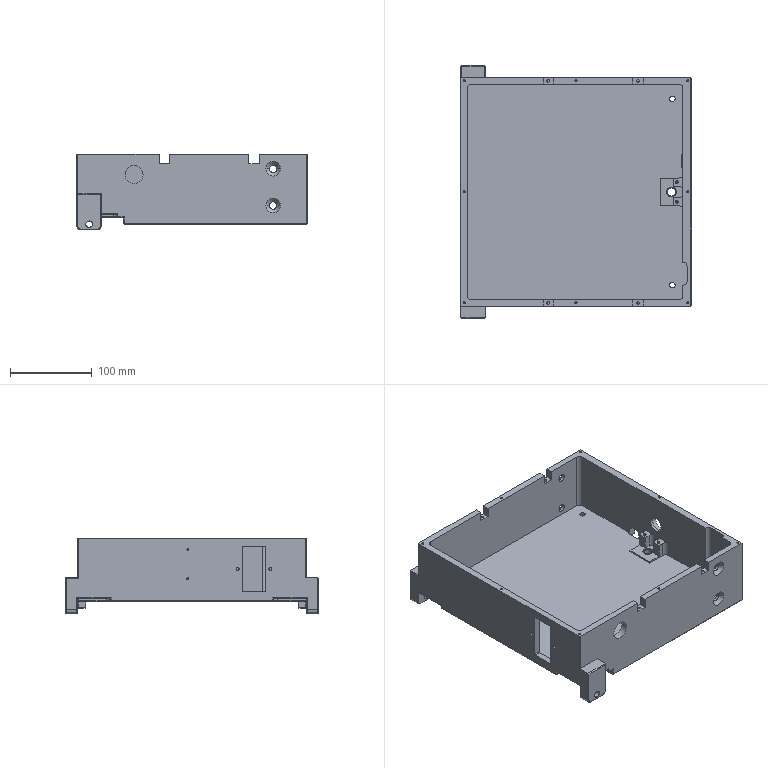CAM job | Mastercam | 3-axis milling, 5-axis milling, drilling
Tools:
tool_number,name,type,diameter_mm,corner_radius_mm,flutes,flute_length_mm,overall_length_mm,shoulder_length_mm,holder_diameter_mm,length_offset,diameter_offset,default_rpm,default_feed_mm_min,default_plunge_mm_min,coolant
1,6 Chamfer Mill,chamfer mill,6,0,4,25,75,30,50,1,1,4167,500.04,600,COOL_OFF
2,2 Flat End Mill,end mill,2,0,4,25,75,25,50,2,2,5000,600,600,COOL_OFF
4,4 Ball Mill / Bull Nose Mill,ball end mill,4,2,4,25,100,30,50,4,4,3000,360,600,COOL_OFF
5,5 Flat End Mill,end mill,5,0,4,25,75,25,50,5,5,2000,240,600,COOL_OFF
6,6 Flat End Mill,end mill,6,0,4,25,75,25,50,6,6,1667,200.04,600,COOL_OFF
7,6 Chamfer Mill,chamfer mill,6,0,4,25,75,30,50,7,7,4167,500.04,600,COOL_OFF
10,10 Flat End Mill,end mill,10,0,4,25,75,25,50,10,10,1000,120,600,COOL_OFF
11,10 Flat End Mill,end mill,10,0,4,25,75,25,50,11,11,1000,120,600,COOL_OFF
12,12 Flat End Mill,end mill,12,0,4,25,75,25,50,12,12,833,99.96,600,COOL_OFF
15,6 Bull Nose Mill,bull end mill,6,1,4,25,100,25,50,15,15,2000,240,600,COOL_OFF
20,20 Flat End Mill,end mill,20,0,4,100,100,100,50,20,20,500,60,600,COOL_OFF
23,50 Flat End Mill,end mill,50,0,4,25,75,25,50,23,23,200,24,600,COOL_OFF
24,100 Flat End Mill,end mill,100,0,4,25,75,25,50,24,24,100,12,600,COOL_OFF
Operations:
seq,operation,operation_type,tool_number,tool_name,tool_diameter_mm,spindle_rpm,feed_mm_min,plunge_mm_min,retract_mm_min,cycle_time_s,wcs,posted,nc_file
1,Facing - [WCS: Plane] - [Tplane: Plane],Facing,24,100 Flat End Mill,100,4000,1200,600,1200,129.734,Plane,yes,.nc
2,Contour (Ramp) - [WCS: Plane] - [Tplane: Plane],Contour,23,50 Flat End Mill,50,4000,4000,600,1200,942.056,Plane,yes,.nc
3,Contour (Ramp) - [WCS: Plane] - [Tplane: Plane],Contour,23,50 Flat End Mill,50,4000,4000,600,1200,945.196,Plane,yes,.nc
4,3D High Speed (Area roughing) - [WCS: Plane] - [Tplane: Plane],HighSpeed3D,23,50 Flat End Mill,50,4000,4000,600,1200,2549.3,Plane,yes,.nc
5,3D High Speed (Waterline rest passes) - [WCS: Plane] - [Tplane: Plane],HighSpeed3D,20,20 Flat End Mill,20,4000,4000,600,1200,319.738,Plane,yes,.nc
6,Contour (Ramp) - [WCS: Plane] - [Tplane: Plane],Contour,10,10 Flat End Mill,10,7000,3000,600,1200,74.419,Plane,yes,.nc
7,Contour (2D) - [WCS: Plane] - [Tplane: Plane],Contour,10,10 Flat End Mill,10,7000,1000,600,1200,25.222,Plane,yes,.nc
8,Contour (2D) - [WCS: Plane] - [Tplane: Plane],Contour,20,20 Flat End Mill,20,4000,2000,600,1200,157.383,Plane,yes,.nc
9,Contour (Remachining) - [WCS: Plane] - [Tplane: Plane],Contour,20,20 Flat End Mill,20,4000,4000,600,1200,81.306,Plane,yes,.nc
10,Contour (2D) - [WCS: Plane] - [Tplane: Plane],Contour,20,20 Flat End Mill,20,4000,2000,600,1200,163.926,Plane,yes,.nc
11,Contour (Remachining) - [WCS: Plane] - [Tplane: Plane],Contour,10,10 Flat End Mill,10,6500,3500,600,1200,145.198,Plane,yes,.nc
12,Contour (2D) - [WCS: Plane] - [Tplane: Plane],Contour,10,10 Flat End Mill,10,6500,1000,600,1200,497.497,Plane,yes,.nc
13,3D High Speed (Waterline rest passes) - [WCS: Plane] - [Tplane: Plane],HighSpeed3D,11,10 Flat End Mill,10,5500,3000,600,1200,255.251,Plane,yes,.nc
14,Contour (2D) - [WCS: Plane] - [Tplane: Plane],Contour,11,10 Flat End Mill,10,5500,1000,600,1200,124.5,Plane,yes,.nc
15,Contour (2D) - [WCS: Plane] - [Tplane: Plane],Contour,11,10 Flat End Mill,10,5500,1000,600,1200,4.343,Plane,yes,.nc
16,2D High Speed (2D Area Mill) - [WCS: Plane] - [Tplane: Plane],HighSpeed2D,11,10 Flat End Mill,10,5500,1000,600,1200,13.176,Plane,yes,.nc
17,Contour (2D) - [WCS: Plane] - [Tplane: Plane],Contour,11,10 Flat End Mill,10,5500,1000,600,1200,22.528,Plane,yes,.nc
18,Contour (2D) - [WCS: Plane] - [Tplane: Plane],Contour,11,10 Flat End Mill,10,5500,1000,600,1200,261.23,Plane,yes,.nc
19,2D High Speed (2D Area Mill) - [WCS: Plane] - [Tplane: Plane],HighSpeed2D,11,10 Flat End Mill,10,5500,1000,600,1200,742.916,Plane,yes,.nc
20,Drill/Counterbore - [WCS: Plane] - [Tplane: Plane],Drill,1,6 Chamfer Mill,6,5000,200,600,1200,15.45,Plane,yes,.nc
21,Contour (2D chamfer) - [WCS: Plane] - [Tplane: Plane],Contour,7,6 Chamfer Mill,6,6000,1200,600,1200,110.416,Plane,yes,.nc
22,Contour (2D chamfer) - [WCS: Plane] - [Tplane: Plane],Contour,7,6 Chamfer Mill,6,6000,1200,600,1200,11.672,Plane,yes,.nc
23,Contour (2D chamfer) - [WCS: Plane] - [Tplane: Plane],Contour,7,6 Chamfer Mill,6,6000,1200,600,1200,15.232,Plane,yes,.nc
24,Facing - [WCS: Plane-1] - [Tplane: Plane-1],Facing,24,100 Flat End Mill,100,4000,2500,600,1200,1022.912,Plane-1,yes,.nc
25,Contour (2D chamfer) - [WCS: Plane-1] - [Tplane: Plane-1],Contour,7,6 Chamfer Mill,6,6000,1200,600,1200,59.589,Plane-1,yes,.nc
26,Manual Entry (G90G54G0X-300.),ManualEntry,,,,0,0,0,0,0,Plane-2,yes,.nc
27,Contour (Ramp) - [WCS: Plane-2] - [Tplane: Plane-2],Contour,10,10 Flat End Mill,10,7000,2500,600,1200,80.177,Plane-2,yes,.nc
28,Manual Entry (G90G54G0X-300.),ManualEntry,,,,0,0,0,0,0,Plane-2,yes,.nc
29,Contour (Remachining) - [WCS: Plane-2] - [Tplane: Plane-2],Contour,2,2 Flat End Mill,2,6000,2000,600,1200,48.112,Plane-2,yes,.nc
30,Contour (Remachining) - [WCS: Plane-2] - [Tplane: Plane-2],Contour,2,2 Flat End Mill,2,6000,500,600,1200,29.929,Plane-2,yes,.nc
31,Manual Entry (G90G54G0X-300.),ManualEntry,,,,0,0,0,0,0,Plane-2,yes,.nc
32,Contour (2D) - [WCS: Plane-2] - [Tplane: Plane-2],Contour,10,10 Flat End Mill,10,7000,1000,600,1200,8.573,Plane-2,yes,.nc
33,Manual Entry (G90G54G0X-300.),ManualEntry,,,,0,0,0,0,0,Plane-2,yes,.nc
34,Drill/Counterbore - [WCS: Plane-2] - [Tplane: Plane-2],Drill,7,6 Chamfer Mill,6,6000,200,600,1200,3.954,Plane-2,yes,.nc
35,Contour (2D chamfer) - [WCS: Plane-2] - [Tplane: Plane-2],Contour,7,6 Chamfer Mill,6,6000,1000,600,1200,10.508,Plane-2,yes,.nc
36,Manual Entry (G90G54G0X-300.),ManualEntry,,,,0,0,0,0,0,Plane-3,yes,.nc
37,Contour (Ramp) - [WCS: Plane-3] - [Tplane: Plane-3],Contour,10,10 Flat End Mill,10,7000,3000,600,1200,55.331,Plane-3,yes,.nc
38,Contour (2D) - [WCS: Plane-3] - [Tplane: Plane-3],Contour,10,10 Flat End Mill,10,7000,1000,600,1200,10.238,Plane-3,yes,.nc
39,Contour (Ramp) - [WCS: Plane-3] - [Tplane: Plane-3],Contour,10,10 Flat End Mill,10,7000,2500,600,1200,13.576,Plane-3,yes,.nc
40,Contour (Ramp) - [WCS: Plane-3] - [Tplane: Plane-3],Contour,10,10 Flat End Mill,10,7000,3000,600,1200,6.513,Plane-3,yes,.nc
41,Contour (2D) - [WCS: Plane-3] - [Tplane: Plane-3],Contour,10,10 Flat End Mill,10,7000,1000,600,1200,3.526,Plane-3,yes,.nc
42,Manual Entry (fbe),ManualEntry,,,,0,0,0,0,0,Plane-3,yes,.nc
43,Contour (2D) - [WCS: Plane-3] - [Tplane: Plane-3],Contour,10,10 Flat End Mill,10,7000,1000,600,1200,6.461,Plane-3,yes,.nc
44,Manual Entry (G90G54G0X-300.),ManualEntry,,,,0,0,0,0,0,Plane-3,yes,.nc
45,Contour (Ramp) - [WCS: Plane-3] - [Tplane: Plane-3],Contour,6,6 Flat End Mill,6,6500,2500,600,1200,12.033,Plane-3,yes,.nc
46,Contour (2D) - [WCS: Plane-3] - [Tplane: Plane-3],Contour,6,6 Flat End Mill,6,6500,1000,600,1200,3.861,Plane-3,yes,.nc
47,Manual Entry (G90G54G0X-300.),ManualEntry,,,,0,0,0,0,0,Plane-3,yes,.nc
48,Contour (2D chamfer) - [WCS: Plane-3] - [Tplane: Plane-3],Contour,7,6 Chamfer Mill,6,6000,1000,600,1200,19.128,Plane-3,yes,.nc
49,Contour (2D chamfer) - [WCS: Plane-3] - [Tplane: Plane-3],Contour,7,6 Chamfer Mill,6,6000,1000,600,1200,8.572,Plane-3,yes,.nc
50,Drill/Counterbore - [WCS: Plane-3] - [Tplane: Plane-3],Drill,7,6 Chamfer Mill,6,6000,200,600,1200,2.966,Plane-3,yes,.nc
51,Manual Entry (G90G54G0X-300.),ManualEntry,,,,0,0,0,0,0,Plane-3,yes,.nc
52,Contour (Ramp) - [WCS: Plane-4] - [Tplane: Plane-4],Contour,12,12 Flat End Mill,12,7000,3000,600,1200,29.857,Plane-4,yes,.nc
53,Contour (Ramp) - [WCS: Plane-4] - [Tplane: Plane-4],Contour,12,12 Flat End Mill,12,7000,3000,600,1200,19.423,Plane-4,yes,.nc
54,Contour (2D) - [WCS: Plane-4] - [Tplane: Plane-4],Contour,12,12 Flat End Mill,12,7000,1000,600,1200,13.482,Plane-4,yes,.nc
55,Manual Entry (G90G54G0X-300.),ManualEntry,,,,0,0,0,0,0,Plane-3,yes,.nc
56,Contour (Ramp) - [WCS: Plane-4] - [Tplane: Plane-4],Contour,5,5 Flat End Mill,5,7000,2500,600,1200,14.495,Plane-4,yes,.nc
57,Contour (Ramp) - [WCS: Plane-4] - [Tplane: Plane-4],Contour,5,5 Flat End Mill,5,7000,1000,600,1200,5.98,Plane-4,yes,.nc
58,Contour (Ramp) - [WCS: Plane-4] - [Tplane: Plane-4],Contour,5,5 Flat End Mill,5,7000,2000,600,1200,11.785,Plane-4,yes,.nc
59,Contour (Ramp) - [WCS: Plane-4] - [Tplane: Plane-4],Contour,5,5 Flat End Mill,5,7000,1000,600,1200,6.231,Plane-4,yes,.nc
60,Manual Entry (G90G54G0X-300.),ManualEntry,,,,0,0,0,0,0,Plane-3,yes,.nc
61,Surface Finish Flowline - [WCS: Plane-4] - [Tplane: Plane-4],MultiSurfaceFinishFlowline,15,6 Bull Nose Mill,6,7000,3000,600,1200,71.4,Plane-4,yes,.nc
62,Manual Entry (G90G54G0X-300.),ManualEntry,,,,0,0,0,0,0,Plane-3,yes,.nc
63,Contour (2D chamfer) - [WCS: Plane-4] - [Tplane: Plane-4],Contour,7,6 Chamfer Mill,6,6000,1000,600,1200,19.072,Plane-4,yes,.nc
64,Contour (2D chamfer) - [WCS: Plane-4] - [Tplane: Plane-4],Contour,7,6 Chamfer Mill,6,6000,1000,600,1200,2.137,Plane-4,yes,.nc
65,Manual Entry (G90G54G0X-300.),ManualEntry,,,,0,0,0,0,0,Plane-3,yes,.nc
66,Contour (Ramp) - [WCS: Plane-5] - [Tplane: Plane-5],Contour,12,12 Flat End Mill,12,7000,3000,600,1200,29.857,Plane-5,yes,.nc
67,Contour (Ramp) - [WCS: Plane-5] - [Tplane: Plane-5],Contour,12,12 Flat End Mill,12,7000,3000,600,1200,19.423,Plane-5,yes,.nc
68,Contour (2D) - [WCS: Plane-5] - [Tplane: Plane-5],Contour,12,12 Flat End Mill,12,7000,1000,600,1200,13.482,Plane-5,yes,.nc
69,Contour (Ramp) - [WCS: Plane-5] - [Tplane: Plane-5],Contour,12,12 Flat End Mill,12,7000,2500,600,1200,12.127,Plane-5,yes,.nc
70,Contour (2D) - [WCS: Plane-5] - [Tplane: Plane-5],Contour,12,12 Flat End Mill,12,7000,1000,600,1200,6.18,Plane-5,yes,.nc
71,Manual Entry (G90G54G0X-300.),ManualEntry,,,,0,0,0,0,0,Plane-3,yes,.nc
72,Contour (Ramp) - [WCS: Plane-5] - [Tplane: Plane-5],Contour,5,5 Flat End Mill,5,7000,2500,600,1200,14.495,Plane-5,yes,.nc
73,Contour (Ramp) - [WCS: Plane-5] - [Tplane: Plane-5],Contour,5,5 Flat End Mill,5,7000,1000,600,1200,5.98,Plane-5,yes,.nc
74,Contour (Ramp) - [WCS: Plane-5] - [Tplane: Plane-5],Contour,5,5 Flat End Mill,5,7000,2000,600,1200,11.785,Plane-5,yes,.nc
75,Contour (Ramp) - [WCS: Plane-5] - [Tplane: Plane-5],Contour,5,5 Flat End Mill,5,7000,1000,600,1200,6.231,Plane-5,yes,.nc
76,Manual Entry (G90G54G0X-300.),ManualEntry,,,,0,0,0,0,0,Plane-3,yes,.nc
77,Surface Finish Flowline - [WCS: Plane-5] - [Tplane: Plane-5],MultiSurfaceFinishFlowline,15,6 Bull Nose Mill,6,7000,3000,600,1200,71.4,Plane-5,yes,.nc
78,Manual Entry (G90G54G0X-300.),ManualEntry,,,,0,0,0,0,0,Plane-3,yes,.nc
79,Contour (2D chamfer) - [WCS: Plane-5] - [Tplane: Plane-5],Contour,7,6 Chamfer Mill,6,6000,1000,600,1200,19.072,Plane-5,yes,.nc
80,Contour (2D chamfer) - [WCS: Plane-5] - [Tplane: Plane-5],Contour,7,6 Chamfer Mill,6,6000,1000,600,1200,7.057,Plane-5,yes,.nc
81,Contour (Ramp) - [WCS: Plane-1] - [Tplane: Plane-1],Contour,23,50 Flat End Mill,50,4000,3500,600,1200,498.753,Plane-1,yes,.nc
82,Contour (Ramp) - [WCS: Plane-1] - [Tplane: Plane-1],Contour,23,50 Flat End Mill,50,4000,3500,600,1200,610.643,Plane-1,yes,.nc
83,2D High Speed (2D Area Mill) - [WCS: Plane-1] - [Tplane: Plane-1],HighSpeed2D,10,10 Flat End Mill,10,7000,4000,600,1200,368.666,Plane-1,yes,.nc
84,Contour (Ramp) - [WCS: Plane-1] - [Tplane: Plane-1],Contour,10,10 Flat End Mill,10,7000,4000,600,1200,10.861,Plane-1,yes,.nc
85,Contour (2D) - [WCS: Plane-1] - [Tplane: Plane-1],Contour,10,10 Flat End Mill,10,7000,800,600,1200,45.535,Plane-1,yes,.nc
86,Contour (2D) - [WCS: Plane-1] - [Tplane: Plane-1],Contour,10,10 Flat End Mill,10,7000,800,600,1200,83.99,Plane-1,yes,.nc
87,Contour (2D) - [WCS: Plane-1] - [Tplane: Plane-1],Contour,10,10 Flat End Mill,10,7000,1000,600,1200,709.438,Plane-1,yes,.nc
88,Contour (2D) - [WCS: Plane-1] - [Tplane: Plane-1],Contour,10,10 Flat End Mill,10,7000,1000,600,1200,24.637,Plane-1,yes,.nc
89,Contour (2D) - [WCS: Plane-1] - [Tplane: Plane-1],Contour,10,10 Flat End Mill,10,7000,1000,600,1200,12.557,Plane-1,yes,.nc
90,Manual Entry (leber),ManualEntry,,,,0,0,0,0,0,Plane-1,yes,.nc
91,Contour (Ramp) - [WCS: Plane-1] - [Tplane: Plane-1],Contour,5,5 Flat End Mill,5,7000,3000,600,1200,6.773,Plane-1,yes,.nc
92,Unified Morph - [WCS: Plane-1] - [Tplane: Plane-1],461,4,4 Ball Mill / Bull Nose Mill,4,7000,3000,600,1200,13.37,Plane-1,yes,.nc
93,Transform/Mirror X Axis/Coordinate/Geometry,XForm,,,,0,0,0,0,13.37,Plane-1,yes,.nc
94,Drill/Counterbore - [WCS: Plane-1] - [Tplane: Plane-1],Drill,7,6 Chamfer Mill,6,6000,200,600,1200,1.977,Plane-1,yes,.nc
95,Contour (2D chamfer) - [WCS: Plane-1] - [Tplane: Plane-1],Contour,7,6 Chamfer Mill,6,6000,1000,600,1200,190.504,Plane-1,yes,.nc
96,Contour (2D chamfer) - [WCS: Plane-1] - [Tplane: Plane-1],Contour,7,6 Chamfer Mill,6,6000,1000,600,1200,10.903,Plane-1,yes,.nc
97,Contour (2D chamfer) - [WCS: Plane-1] - [Tplane: Plane-1],Contour,7,6 Chamfer Mill,6,6000,1000,600,1200,15.428,Plane-1,yes,.nc
98,Contour (2D chamfer) - [WCS: Plane-1] - [Tplane: Plane-1],Contour,7,6 Chamfer Mill,6,6000,1000,600,1200,11.559,Plane-1,yes,.nc